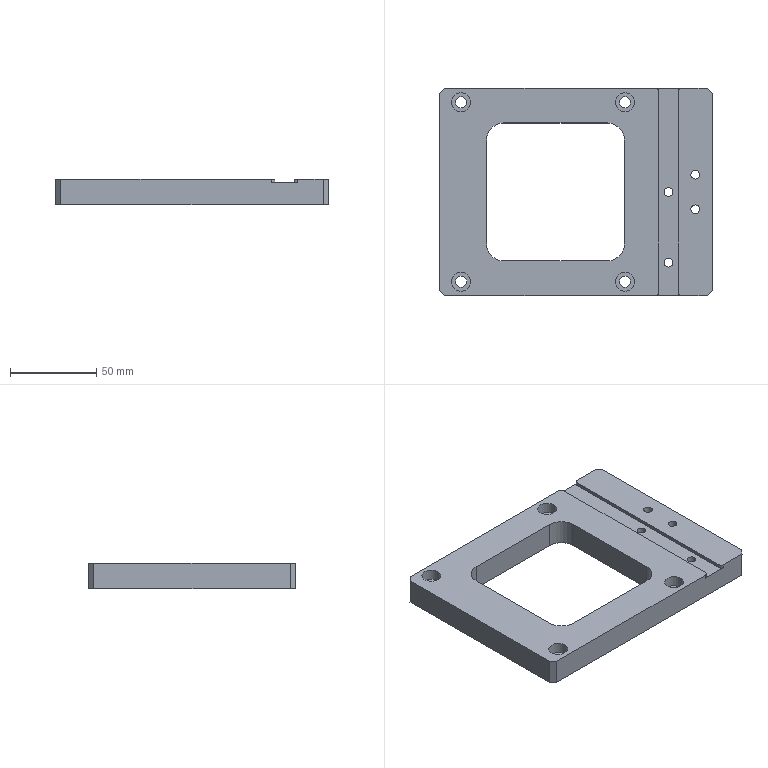Part | 1 solid | 42 faces | box 158.2 x 120 x 15 mm | volume 182408 mm3 | plane 22 | cylinder 20 | commonest cylinder face diameters 4 x4 5 x4 6.5 x4 11 x4 20 x4
STEP:
#1=CARTESIAN_POINT('',(62.95,-354.903,303.7));
#2=VERTEX_POINT('',#1);
#3=CARTESIAN_POINT('',(60.95,-352.903,303.7));
#4=VERTEX_POINT('',#3);
#5=CARTESIAN_POINT('',(60.95,-354.903,303.7));
#6=DIRECTION('',(0.,-0.000000076,1.));
#7=DIRECTION('',(0.,-1.,-0.000000076));
#8=AXIS2_PLACEMENT_3D('',#5,#6,#7);
#9=CIRCLE('',#8,2.);
#10=EDGE_CURVE('',#2,#4,#9,.T.);
#11=ORIENTED_EDGE('',*,*,#10,.F.);
#12=CARTESIAN_POINT('',(62.95,-354.903,301.7));
#13=VERTEX_POINT('',#12);
#14=CARTESIAN_POINT('',(62.95,-354.903,301.7));
#15=DIRECTION('',(0.,0.000000076,-1.));
#16=VECTOR('',#15,1000.);
#17=LINE('',#14,#16);
#18=EDGE_CURVE('',#2,#13,#17,.T.);
#19=ORIENTED_EDGE('',*,*,#18,.T.);
#20=CARTESIAN_POINT('',(60.95,-352.903,301.7));
#21=VERTEX_POINT('',#20);
#22=CARTESIAN_POINT('',(60.95,-354.903,301.7));
#23=DIRECTION('',(0.,-0.000000076,1.));
#24=DIRECTION('',(0.,1.,0.000000076));
#25=AXIS2_PLACEMENT_3D('',#22,#23,#24);
#26=CIRCLE('',#25,2.);
#27=EDGE_CURVE('',#13,#21,#26,.T.);
#28=ORIENTED_EDGE('',*,*,#27,.T.);
#29=CARTESIAN_POINT('',(60.95,-352.903,300.7));
#30=DIRECTION('',(0.,-0.000000076,1.));
#31=VECTOR('',#30,1000.);
#32=LINE('',#29,#31);
#33=EDGE_CURVE('',#21,#4,#32,.T.);
#34=ORIENTED_EDGE('',*,*,#33,.T.);
#35=EDGE_LOOP('',(#11,#19,#28,#34));
#36=FACE_BOUND('',#35,.T.);
#37=CARTESIAN_POINT('',(60.95,-354.903,300.7));
#38=DIRECTION('',(0.,0.000000076,-1.));
#39=DIRECTION('',(0.,1.,0.000000076));
#40=AXIS2_PLACEMENT_3D('',#37,#38,#39);
#41=CYLINDRICAL_SURFACE('',#40,2.);
#42=ADVANCED_FACE('',(#36),#41,.T.);
#43=ORIENTED_EDGE('',*,*,#18,.F.);
#44=CARTESIAN_POINT('',(62.95,-470.903,303.7));
#45=VERTEX_POINT('',#44);
#46=CARTESIAN_POINT('',(62.95,-546.403,303.7));
#47=DIRECTION('',(0.,-1.,-0.000000076));
#48=VECTOR('',#47,1000.);
#49=LINE('',#46,#48);
#50=EDGE_CURVE('',#2,#45,#49,.T.);
#51=ORIENTED_EDGE('',*,*,#50,.T.);
#52=CARTESIAN_POINT('',(62.95,-470.903,301.7));
#53=VERTEX_POINT('',#52);
#54=CARTESIAN_POINT('',(62.95,-470.903,301.7));
#55=DIRECTION('',(0.,-0.000000076,1.));
#56=VECTOR('',#55,1000.);
#57=LINE('',#54,#56);
#58=EDGE_CURVE('',#53,#45,#57,.T.);
#59=ORIENTED_EDGE('',*,*,#58,.F.);
#60=CARTESIAN_POINT('',(62.95,-412.903,301.7));
#61=DIRECTION('',(0.,-1.,-0.000000076));
#62=VECTOR('',#61,1000.);
#63=LINE('',#60,#62);
#64=EDGE_CURVE('',#13,#53,#63,.T.);
#65=ORIENTED_EDGE('',*,*,#64,.F.);
#66=EDGE_LOOP('',(#43,#51,#59,#65));
#67=FACE_BOUND('',#66,.T.);
#68=CARTESIAN_POINT('',(62.95,-432.903,301.7));
#69=DIRECTION('',(-1.,0.,0.));
#70=DIRECTION('',(0.,0.000000051,-1.));
#71=AXIS2_PLACEMENT_3D('',#68,#69,#70);
#72=PLANE('',#71);
#73=ADVANCED_FACE('',(#67),#72,.F.);
#74=CARTESIAN_POINT('',(60.95,-472.903,303.7));
#75=VERTEX_POINT('',#74);
#76=CARTESIAN_POINT('',(60.95,-470.903,303.7));
#77=DIRECTION('',(0.,-0.000000076,1.));
#78=DIRECTION('',(0.,-1.,-0.000000076));
#79=AXIS2_PLACEMENT_3D('',#76,#77,#78);
#80=CIRCLE('',#79,2.);
#81=EDGE_CURVE('',#75,#45,#80,.T.);
#82=ORIENTED_EDGE('',*,*,#81,.F.);
#83=CARTESIAN_POINT('',(60.95,-472.903,301.7));
#84=VERTEX_POINT('',#83);
#85=CARTESIAN_POINT('',(60.95,-472.903,288.7));
#86=DIRECTION('',(0.,0.000000076,-1.));
#87=VECTOR('',#86,1000.);
#88=LINE('',#85,#87);
#89=EDGE_CURVE('',#75,#84,#88,.T.);
#90=ORIENTED_EDGE('',*,*,#89,.T.);
#91=CARTESIAN_POINT('',(60.95,-470.903,301.7));
#92=DIRECTION('',(0.,-0.000000076,1.));
#93=DIRECTION('',(0.,1.,0.000000076));
#94=AXIS2_PLACEMENT_3D('',#91,#92,#93);
#95=CIRCLE('',#94,2.);
#96=EDGE_CURVE('',#84,#53,#95,.T.);
#97=ORIENTED_EDGE('',*,*,#96,.T.);
#98=ORIENTED_EDGE('',*,*,#58,.T.);
#99=EDGE_LOOP('',(#82,#90,#97,#98));
#100=FACE_BOUND('',#99,.T.);
#101=CARTESIAN_POINT('',(60.95,-470.903,288.7));
#102=DIRECTION('',(0.,-0.000000076,1.));
#103=DIRECTION('',(0.,-1.,-0.000000076));
#104=AXIS2_PLACEMENT_3D('',#101,#102,#103);
#105=CYLINDRICAL_SURFACE('',#104,2.);
#106=ADVANCED_FACE('',(#100),#105,.T.);
#107=ORIENTED_EDGE('',*,*,#89,.F.);
#108=CARTESIAN_POINT('',(-61.2,-472.903,303.7));
#109=VERTEX_POINT('',#108);
#110=CARTESIAN_POINT('',(3.,-472.903,303.7));
#111=DIRECTION('',(-1.,0.,0.));
#112=VECTOR('',#111,1000.);
#113=LINE('',#110,#112);
#114=EDGE_CURVE('',#75,#109,#113,.T.);
#115=ORIENTED_EDGE('',*,*,#114,.T.);
#116=CARTESIAN_POINT('',(-61.2,-472.903,288.7));
#117=VERTEX_POINT('',#116);
#118=CARTESIAN_POINT('',(-61.2,-472.903,288.7));
#119=DIRECTION('',(0.,-0.000000076,1.));
#120=VECTOR('',#119,1000.);
#121=LINE('',#118,#120);
#122=EDGE_CURVE('',#117,#109,#121,.T.);
#123=ORIENTED_EDGE('',*,*,#122,.F.);
#124=CARTESIAN_POINT('',(91.,-472.903,288.7));
#125=VERTEX_POINT('',#124);
#126=CARTESIAN_POINT('',(3.,-472.903,288.7));
#127=DIRECTION('',(1.,0.,0.));
#128=VECTOR('',#127,1000.);
#129=LINE('',#126,#128);
#130=EDGE_CURVE('',#117,#125,#129,.T.);
#131=ORIENTED_EDGE('',*,*,#130,.T.);
#132=CARTESIAN_POINT('',(91.,-472.903,303.7));
#133=VERTEX_POINT('',#132);
#134=CARTESIAN_POINT('',(91.,-472.903,288.7));
#135=DIRECTION('',(0.,0.000000076,-1.));
#136=VECTOR('',#135,1000.);
#137=LINE('',#134,#136);
#138=EDGE_CURVE('',#133,#125,#137,.T.);
#139=ORIENTED_EDGE('',*,*,#138,.F.);
#140=CARTESIAN_POINT('',(76.05,-472.903,303.7));
#141=VERTEX_POINT('',#140);
#142=CARTESIAN_POINT('',(-67.,-472.903,303.7));
#143=DIRECTION('',(1.,0.,0.));
#144=VECTOR('',#143,1000.);
#145=LINE('',#142,#144);
#146=EDGE_CURVE('',#141,#133,#145,.T.);
#147=ORIENTED_EDGE('',*,*,#146,.F.);
#148=CARTESIAN_POINT('',(76.05,-472.903,301.7));
#149=VERTEX_POINT('',#148);
#150=CARTESIAN_POINT('',(76.05,-472.903,288.7));
#151=DIRECTION('',(0.,-0.000000076,1.));
#152=VECTOR('',#151,1000.);
#153=LINE('',#150,#152);
#154=EDGE_CURVE('',#149,#141,#153,.T.);
#155=ORIENTED_EDGE('',*,*,#154,.F.);
#156=CARTESIAN_POINT('',(68.5,-472.903,301.7));
#157=DIRECTION('',(1.,0.,0.));
#158=VECTOR('',#157,1000.);
#159=LINE('',#156,#158);
#160=EDGE_CURVE('',#84,#149,#159,.T.);
#161=ORIENTED_EDGE('',*,*,#160,.F.);
#162=EDGE_LOOP('',(#107,#115,#123,#131,#139,#147,#155,#161));
#163=FACE_BOUND('',#162,.T.);
#164=CARTESIAN_POINT('',(-67.,-472.903,288.7));
#165=DIRECTION('',(0.,1.,0.000000076));
#166=DIRECTION('',(1.,0.,0.));
#167=AXIS2_PLACEMENT_3D('',#164,#165,#166);
#168=PLANE('',#167);
#169=ADVANCED_FACE('',(#163),#168,.F.);
#170=ORIENTED_EDGE('',*,*,#122,.T.);
#171=CARTESIAN_POINT('',(-64.2,-469.903,303.7));
#172=VERTEX_POINT('',#171);
#173=CARTESIAN_POINT('',(7.65,-541.753,303.7));
#174=DIRECTION('',(-0.7071,0.7071,0.000000054));
#175=VECTOR('',#174,1000.);
#176=LINE('',#173,#175);
#177=EDGE_CURVE('',#109,#172,#176,.T.);
#178=ORIENTED_EDGE('',*,*,#177,.T.);
#179=CARTESIAN_POINT('',(-64.2,-469.903,288.7));
#180=VERTEX_POINT('',#179);
#181=CARTESIAN_POINT('',(-64.2,-469.903,300.7));
#182=DIRECTION('',(0.,0.000000076,-1.));
#183=VECTOR('',#182,1000.);
#184=LINE('',#181,#183);
#185=EDGE_CURVE('',#172,#180,#184,.T.);
#186=ORIENTED_EDGE('',*,*,#185,.T.);
#187=CARTESIAN_POINT('',(-64.2,-469.903,288.7));
#188=DIRECTION('',(0.7071,-0.7071,-0.000000054));
#189=VECTOR('',#188,1000.);
#190=LINE('',#187,#189);
#191=EDGE_CURVE('',#180,#117,#190,.T.);
#192=ORIENTED_EDGE('',*,*,#191,.T.);
#193=EDGE_LOOP('',(#170,#178,#186,#192));
#194=FACE_BOUND('',#193,.T.);
#195=CARTESIAN_POINT('',(-64.2,-469.903,300.7));
#196=DIRECTION('',(0.7071,0.7071,0.000000054));
#197=DIRECTION('',(0.,-0.000000076,1.));
#198=AXIS2_PLACEMENT_3D('',#195,#196,#197);
#199=PLANE('',#198);
#200=ADVANCED_FACE('',(#194),#199,.F.);
#201=ORIENTED_EDGE('',*,*,#185,.F.);
#202=CARTESIAN_POINT('',(-64.2,-355.903,303.7));
#203=VERTEX_POINT('',#202);
#204=CARTESIAN_POINT('',(-64.2,-546.403,303.7));
#205=DIRECTION('',(0.,1.,0.000000076));
#206=VECTOR('',#205,1000.);
#207=LINE('',#204,#206);
#208=EDGE_CURVE('',#172,#203,#207,.T.);
#209=ORIENTED_EDGE('',*,*,#208,.T.);
#210=CARTESIAN_POINT('',(-64.2,-355.903,288.7));
#211=VERTEX_POINT('',#210);
#212=CARTESIAN_POINT('',(-64.2,-355.903,300.7));
#213=DIRECTION('',(0.,-0.000000076,1.));
#214=VECTOR('',#213,1000.);
#215=LINE('',#212,#214);
#216=EDGE_CURVE('',#211,#203,#215,.T.);
#217=ORIENTED_EDGE('',*,*,#216,.F.);
#218=CARTESIAN_POINT('',(-64.2,-746.403,288.7));
#219=DIRECTION('',(0.,1.,0.000000076));
#220=VECTOR('',#219,1000.);
#221=LINE('',#218,#220);
#222=EDGE_CURVE('',#180,#211,#221,.T.);
#223=ORIENTED_EDGE('',*,*,#222,.F.);
#224=EDGE_LOOP('',(#201,#209,#217,#223));
#225=FACE_BOUND('',#224,.T.);
#226=CARTESIAN_POINT('',(-64.2,-746.403,300.7));
#227=DIRECTION('',(1.,0.,0.));
#228=DIRECTION('',(0.,-0.000000076,1.));
#229=AXIS2_PLACEMENT_3D('',#226,#227,#228);
#230=PLANE('',#229);
#231=ADVANCED_FACE('',(#225),#230,.F.);
#232=ORIENTED_EDGE('',*,*,#216,.T.);
#233=CARTESIAN_POINT('',(-61.2,-352.903,303.7));
#234=VERTEX_POINT('',#233);
#235=CARTESIAN_POINT('',(-125.85,-417.553,303.7));
#236=DIRECTION('',(0.7071,0.7071,0.000000054));
#237=VECTOR('',#236,1000.);
#238=LINE('',#235,#237);
#239=EDGE_CURVE('',#203,#234,#238,.T.);
#240=ORIENTED_EDGE('',*,*,#239,.T.);
#241=CARTESIAN_POINT('',(-61.2,-352.903,288.7));
#242=VERTEX_POINT('',#241);
#243=CARTESIAN_POINT('',(-61.2,-352.903,300.7));
#244=DIRECTION('',(0.,0.000000076,-1.));
#245=VECTOR('',#244,1000.);
#246=LINE('',#243,#245);
#247=EDGE_CURVE('',#234,#242,#246,.T.);
#248=ORIENTED_EDGE('',*,*,#247,.T.);
#249=CARTESIAN_POINT('',(-64.2,-355.903,288.7));
#250=DIRECTION('',(-0.7071,-0.7071,-0.000000054));
#251=VECTOR('',#250,1000.);
#252=LINE('',#249,#251);
#253=EDGE_CURVE('',#242,#211,#252,.T.);
#254=ORIENTED_EDGE('',*,*,#253,.T.);
#255=EDGE_LOOP('',(#232,#240,#248,#254));
#256=FACE_BOUND('',#255,.T.);
#257=CARTESIAN_POINT('',(-64.2,-355.903,300.7));
#258=DIRECTION('',(0.7071,-0.7071,-0.000000054));
#259=DIRECTION('',(0.,0.000000076,-1.));
#260=AXIS2_PLACEMENT_3D('',#257,#258,#259);
#261=PLANE('',#260);
#262=ADVANCED_FACE('',(#256),#261,.F.);
#263=ORIENTED_EDGE('',*,*,#247,.F.);
#264=CARTESIAN_POINT('',(3.,-352.903,303.7));
#265=DIRECTION('',(1.,0.,0.));
#266=VECTOR('',#265,1000.);
#267=LINE('',#264,#266);
#268=EDGE_CURVE('',#234,#4,#267,.T.);
#269=ORIENTED_EDGE('',*,*,#268,.T.);
#270=ORIENTED_EDGE('',*,*,#33,.F.);
#271=CARTESIAN_POINT('',(76.05,-352.903,301.7));
#272=VERTEX_POINT('',#271);
#273=CARTESIAN_POINT('',(68.5,-352.903,301.7));
#274=DIRECTION('',(-1.,0.,0.));
#275=VECTOR('',#274,1000.);
#276=LINE('',#273,#275);
#277=EDGE_CURVE('',#272,#21,#276,.T.);
#278=ORIENTED_EDGE('',*,*,#277,.F.);
#279=CARTESIAN_POINT('',(76.05,-352.903,303.7));
#280=VERTEX_POINT('',#279);
#281=CARTESIAN_POINT('',(76.05,-352.903,300.7));
#282=DIRECTION('',(0.,0.000000076,-1.));
#283=VECTOR('',#282,1000.);
#284=LINE('',#281,#283);
#285=EDGE_CURVE('',#280,#272,#284,.T.);
#286=ORIENTED_EDGE('',*,*,#285,.F.);
#287=CARTESIAN_POINT('',(91.,-352.903,303.7));
#288=VERTEX_POINT('',#287);
#289=CARTESIAN_POINT('',(-67.,-352.903,303.7));
#290=DIRECTION('',(-1.,0.,0.));
#291=VECTOR('',#290,1000.);
#292=LINE('',#289,#291);
#293=EDGE_CURVE('',#288,#280,#292,.T.);
#294=ORIENTED_EDGE('',*,*,#293,.F.);
#295=CARTESIAN_POINT('',(91.,-352.903,288.7));
#296=VERTEX_POINT('',#295);
#297=CARTESIAN_POINT('',(91.,-352.903,300.7));
#298=DIRECTION('',(0.,-0.000000076,1.));
#299=VECTOR('',#298,1000.);
#300=LINE('',#297,#299);
#301=EDGE_CURVE('',#296,#288,#300,.T.);
#302=ORIENTED_EDGE('',*,*,#301,.F.);
#303=CARTESIAN_POINT('',(-67.,-352.903,288.7));
#304=DIRECTION('',(1.,0.,0.));
#305=VECTOR('',#304,1000.);
#306=LINE('',#303,#305);
#307=EDGE_CURVE('',#242,#296,#306,.T.);
#308=ORIENTED_EDGE('',*,*,#307,.F.);
#309=EDGE_LOOP('',(#263,#269,#270,#278,#286,#294,#302,#308));
#310=FACE_BOUND('',#309,.T.);
#311=CARTESIAN_POINT('',(-67.,-352.903,300.7));
#312=DIRECTION('',(0.,-1.,-0.000000076));
#313=DIRECTION('',(0.,0.000000076,-1.));
#314=AXIS2_PLACEMENT_3D('',#311,#312,#313);
#315=PLANE('',#314);
#316=ADVANCED_FACE('',(#310),#315,.F.);
#317=CARTESIAN_POINT('',(84.,-405.403,303.7));
#318=VERTEX_POINT('',#317);
#319=CARTESIAN_POINT('',(84.,-402.903,303.7));
#320=DIRECTION('',(0.,0.000000076,-1.));
#321=DIRECTION('',(0.,-1.,-0.000000076));
#322=AXIS2_PLACEMENT_3D('',#319,#320,#321);
#323=CIRCLE('',#322,2.5);
#324=EDGE_CURVE('',#318,#318,#323,.T.);
#325=ORIENTED_EDGE('',*,*,#324,.T.);
#326=EDGE_LOOP('',(#325));
#327=FACE_BOUND('',#326,.T.);
#328=CARTESIAN_POINT('',(84.,-425.403,303.7));
#329=VERTEX_POINT('',#328);
#330=CARTESIAN_POINT('',(84.,-422.903,303.7));
#331=DIRECTION('',(0.,0.000000076,-1.));
#332=DIRECTION('',(0.,-1.,-0.000000076));
#333=AXIS2_PLACEMENT_3D('',#330,#331,#332);
#334=CIRCLE('',#333,2.5);
#335=EDGE_CURVE('',#329,#329,#334,.T.);
#336=ORIENTED_EDGE('',*,*,#335,.T.);
#337=EDGE_LOOP('',(#336));
#338=FACE_BOUND('',#337,.T.);
#339=CARTESIAN_POINT('',(74.05,-354.903,303.7));
#340=VERTEX_POINT('',#339);
#341=CARTESIAN_POINT('',(76.05,-354.903,303.7));
#342=DIRECTION('',(0.,-0.000000076,1.));
#343=DIRECTION('',(0.,-1.,-0.000000076));
#344=AXIS2_PLACEMENT_3D('',#341,#342,#343);
#345=CIRCLE('',#344,2.);
#346=EDGE_CURVE('',#340,#280,#345,.F.);
#347=ORIENTED_EDGE('',*,*,#346,.F.);
#348=CARTESIAN_POINT('',(74.05,-470.903,303.7));
#349=VERTEX_POINT('',#348);
#350=CARTESIAN_POINT('',(74.05,-432.903,303.7));
#351=DIRECTION('',(0.,-1.,-0.000000076));
#352=VECTOR('',#351,1000.);
#353=LINE('',#350,#352);
#354=EDGE_CURVE('',#340,#349,#353,.T.);
#355=ORIENTED_EDGE('',*,*,#354,.T.);
#356=CARTESIAN_POINT('',(76.05,-470.903,303.7));
#357=DIRECTION('',(0.,-0.000000076,1.));
#358=DIRECTION('',(0.,-1.,-0.000000076));
#359=AXIS2_PLACEMENT_3D('',#356,#357,#358);
#360=CIRCLE('',#359,2.);
#361=EDGE_CURVE('',#141,#349,#360,.F.);
#362=ORIENTED_EDGE('',*,*,#361,.F.);
#363=ORIENTED_EDGE('',*,*,#146,.T.);
#364=CARTESIAN_POINT('',(94.,-469.903,303.7));
#365=VERTEX_POINT('',#364);
#366=CARTESIAN_POINT('',(91.,-472.903,303.7));
#367=DIRECTION('',(0.7071,0.7071,0.000000054));
#368=VECTOR('',#367,1000.);
#369=LINE('',#366,#368);
#370=EDGE_CURVE('',#133,#365,#369,.T.);
#371=ORIENTED_EDGE('',*,*,#370,.T.);
#372=CARTESIAN_POINT('',(94.,-355.903,303.7));
#373=VERTEX_POINT('',#372);
#374=CARTESIAN_POINT('',(94.,-450.403,303.7));
#375=DIRECTION('',(0.,1.,0.000000076));
#376=VECTOR('',#375,1000.);
#377=LINE('',#374,#376);
#378=EDGE_CURVE('',#365,#373,#377,.T.);
#379=ORIENTED_EDGE('',*,*,#378,.T.);
#380=CARTESIAN_POINT('',(91.,-352.903,303.7));
#381=DIRECTION('',(-0.7071,0.7071,0.000000054));
#382=VECTOR('',#381,1000.);
#383=LINE('',#380,#382);
#384=EDGE_CURVE('',#373,#288,#383,.T.);
#385=ORIENTED_EDGE('',*,*,#384,.T.);
#386=ORIENTED_EDGE('',*,*,#293,.T.);
#387=EDGE_LOOP('',(#347,#355,#362,#363,#371,#379,#385,#386));
#388=FACE_BOUND('',#387,.T.);
#389=CARTESIAN_POINT('',(3.,-546.403,303.7));
#390=DIRECTION('',(0.,-0.000000076,1.));
#391=DIRECTION('',(0.,-1.,-0.000000076));
#392=AXIS2_PLACEMENT_3D('',#389,#390,#391);
#393=PLANE('',#392);
#394=ADVANCED_FACE('',(#327,#338,#388),#393,.T.);
#395=CARTESIAN_POINT('',(84.,-405.403,288.7));
#396=VERTEX_POINT('',#395);
#397=CARTESIAN_POINT('',(84.,-402.903,288.7));
#398=DIRECTION('',(0.,0.000000076,-1.));
#399=DIRECTION('',(0.,-1.,-0.000000076));
#400=AXIS2_PLACEMENT_3D('',#397,#398,#399);
#401=CIRCLE('',#400,2.5);
#402=EDGE_CURVE('',#396,#396,#401,.T.);
#403=ORIENTED_EDGE('',*,*,#402,.T.);
#404=EDGE_LOOP('',(#403));
#405=FACE_BOUND('',#404,.T.);
#406=ORIENTED_EDGE('',*,*,#324,.F.);
#407=EDGE_LOOP('',(#406));
#408=FACE_BOUND('',#407,.T.);
#409=CARTESIAN_POINT('',(84.,-402.903,296.2));
#410=DIRECTION('',(0.,0.000000076,-1.));
#411=DIRECTION('',(1.,0.,0.));
#412=AXIS2_PLACEMENT_3D('',#409,#410,#411);
#413=CYLINDRICAL_SURFACE('',#412,2.5);
#414=ADVANCED_FACE('',(#405,#408),#413,.F.);
#415=CARTESIAN_POINT('',(84.,-425.403,288.7));
#416=VERTEX_POINT('',#415);
#417=CARTESIAN_POINT('',(84.,-422.903,288.7));
#418=DIRECTION('',(0.,0.000000076,-1.));
#419=DIRECTION('',(0.,-1.,-0.000000076));
#420=AXIS2_PLACEMENT_3D('',#417,#418,#419);
#421=CIRCLE('',#420,2.5);
#422=EDGE_CURVE('',#416,#416,#421,.T.);
#423=ORIENTED_EDGE('',*,*,#422,.T.);
#424=EDGE_LOOP('',(#423));
#425=FACE_BOUND('',#424,.T.);
#426=ORIENTED_EDGE('',*,*,#335,.F.);
#427=EDGE_LOOP('',(#426));
#428=FACE_BOUND('',#427,.T.);
#429=CARTESIAN_POINT('',(84.,-422.903,296.2));
#430=DIRECTION('',(0.,0.000000076,-1.));
#431=DIRECTION('',(1.,0.,0.));
#432=AXIS2_PLACEMENT_3D('',#429,#430,#431);
#433=CYLINDRICAL_SURFACE('',#432,2.5);
#434=ADVANCED_FACE('',(#425,#428),#433,.F.);
#435=ORIENTED_EDGE('',*,*,#154,.T.);
#436=ORIENTED_EDGE('',*,*,#361,.T.);
#437=CARTESIAN_POINT('',(74.05,-470.903,301.7));
#438=VERTEX_POINT('',#437);
#439=CARTESIAN_POINT('',(74.05,-470.903,301.7));
#440=DIRECTION('',(0.,0.000000076,-1.));
#441=VECTOR('',#440,1000.);
#442=LINE('',#439,#441);
#443=EDGE_CURVE('',#349,#438,#442,.T.);
#444=ORIENTED_EDGE('',*,*,#443,.T.);
#445=CARTESIAN_POINT('',(76.05,-470.903,301.7));
#446=DIRECTION('',(0.,-0.000000076,1.));
#447=DIRECTION('',(0.,1.,0.000000076));
#448=AXIS2_PLACEMENT_3D('',#445,#446,#447);
#449=CIRCLE('',#448,2.);
#450=EDGE_CURVE('',#438,#149,#449,.T.);
#451=ORIENTED_EDGE('',*,*,#450,.T.);
#452=EDGE_LOOP('',(#435,#436,#444,#451));
#453=FACE_BOUND('',#452,.T.);
#454=CARTESIAN_POINT('',(76.05,-470.903,288.7));
#455=DIRECTION('',(0.,0.000000076,-1.));
#456=DIRECTION('',(0.,1.,0.000000076));
#457=AXIS2_PLACEMENT_3D('',#454,#455,#456);
#458=CYLINDRICAL_SURFACE('',#457,2.);
#459=ADVANCED_FACE('',(#453),#458,.T.);
#460=CARTESIAN_POINT('',(74.05,-354.903,301.7));
#461=VERTEX_POINT('',#460);
#462=CARTESIAN_POINT('',(74.05,-354.903,301.7));
#463=DIRECTION('',(0.,-0.000000076,1.));
#464=VECTOR('',#463,1000.);
#465=LINE('',#462,#464);
#466=EDGE_CURVE('',#461,#340,#465,.T.);
#467=ORIENTED_EDGE('',*,*,#466,.T.);
#468=ORIENTED_EDGE('',*,*,#346,.T.);
#469=ORIENTED_EDGE('',*,*,#285,.T.);
#470=CARTESIAN_POINT('',(76.05,-354.903,301.7));
#471=DIRECTION('',(0.,-0.000000076,1.));
#472=DIRECTION('',(0.,1.,0.000000076));
#473=AXIS2_PLACEMENT_3D('',#470,#471,#472);
#474=CIRCLE('',#473,2.);
#475=EDGE_CURVE('',#272,#461,#474,.T.);
#476=ORIENTED_EDGE('',*,*,#475,.T.);
#477=EDGE_LOOP('',(#467,#468,#469,#476));
#478=FACE_BOUND('',#477,.T.);
#479=CARTESIAN_POINT('',(76.05,-354.903,300.7));
#480=DIRECTION('',(0.,-0.000000076,1.));
#481=DIRECTION('',(0.,-1.,-0.000000076));
#482=AXIS2_PLACEMENT_3D('',#479,#480,#481);
#483=CYLINDRICAL_SURFACE('',#482,2.);
#484=ADVANCED_FACE('',(#478),#483,.T.);
#485=CARTESIAN_POINT('',(33.,-452.903,288.7));
#486=VERTEX_POINT('',#485);
#487=CARTESIAN_POINT('',(33.,-452.903,303.7));
#488=VERTEX_POINT('',#487);
#489=CARTESIAN_POINT('',(33.,-452.903,296.2));
#490=DIRECTION('',(0.,-0.000000076,1.));
#491=VECTOR('',#490,1000.);
#492=LINE('',#489,#491);
#493=EDGE_CURVE('',#486,#488,#492,.T.);
#494=ORIENTED_EDGE('',*,*,#493,.T.);
#495=CARTESIAN_POINT('',(43.,-442.903,303.7));
#496=VERTEX_POINT('',#495);
#497=CARTESIAN_POINT('',(33.,-442.903,303.7));
#498=DIRECTION('',(0.,-0.000000076,1.));
#499=DIRECTION('',(0.,-1.,-0.000000076));
#500=AXIS2_PLACEMENT_3D('',#497,#498,#499);
#501=CIRCLE('',#500,10.);
#502=EDGE_CURVE('',#488,#496,#501,.T.);
#503=ORIENTED_EDGE('',*,*,#502,.T.);
#504=CARTESIAN_POINT('',(43.,-442.903,288.7));
#505=VERTEX_POINT('',#504);
#506=CARTESIAN_POINT('',(43.,-442.903,303.7));
#507=DIRECTION('',(0.,0.000000076,-1.));
#508=VECTOR('',#507,1000.);
#509=LINE('',#506,#508);
#510=EDGE_CURVE('',#496,#505,#509,.T.);
#511=ORIENTED_EDGE('',*,*,#510,.T.);
#512=CARTESIAN_POINT('',(33.,-442.903,288.7));
#513=DIRECTION('',(0.,0.000000076,-1.));
#514=DIRECTION('',(0.,-1.,-0.000000076));
#515=AXIS2_PLACEMENT_3D('',#512,#513,#514);
#516=CIRCLE('',#515,10.);
#517=EDGE_CURVE('',#505,#486,#516,.T.);
#518=ORIENTED_EDGE('',*,*,#517,.T.);
#519=EDGE_LOOP('',(#494,#503,#511,#518));
#520=FACE_BOUND('',#519,.T.);
#521=CARTESIAN_POINT('',(33.,-442.903,303.7));
#522=DIRECTION('',(0.,-0.000000076,1.));
#523=DIRECTION('',(0.,-1.,-0.000000076));
#524=AXIS2_PLACEMENT_3D('',#521,#522,#523);
#525=CYLINDRICAL_SURFACE('',#524,10.);
#526=ADVANCED_FACE('',(#520),#525,.F.);
#527=CARTESIAN_POINT('',(-37.,-442.903,288.7));
#528=VERTEX_POINT('',#527);
#529=CARTESIAN_POINT('',(-37.,-442.903,303.7));
#530=VERTEX_POINT('',#529);
#531=CARTESIAN_POINT('',(-37.,-442.903,288.7));
#532=DIRECTION('',(0.,-0.000000076,1.));
#533=VECTOR('',#532,1000.);
#534=LINE('',#531,#533);
#535=EDGE_CURVE('',#528,#530,#534,.T.);
#536=ORIENTED_EDGE('',*,*,#535,.T.);
#537=CARTESIAN_POINT('',(-27.,-452.903,303.7));
#538=VERTEX_POINT('',#537);
#539=CARTESIAN_POINT('',(-27.,-442.903,303.7));
#540=DIRECTION('',(0.,-0.000000076,1.));
#541=DIRECTION('',(0.,-1.,-0.000000076));
#542=AXIS2_PLACEMENT_3D('',#539,#540,#541);
#543=CIRCLE('',#542,10.);
#544=EDGE_CURVE('',#530,#538,#543,.T.);
#545=ORIENTED_EDGE('',*,*,#544,.T.);
#546=CARTESIAN_POINT('',(-27.,-452.903,288.7));
#547=VERTEX_POINT('',#546);
#548=CARTESIAN_POINT('',(-27.,-452.903,303.7));
#549=DIRECTION('',(0.,0.000000076,-1.));
#550=VECTOR('',#549,1000.);
#551=LINE('',#548,#550);
#552=EDGE_CURVE('',#538,#547,#551,.T.);
#553=ORIENTED_EDGE('',*,*,#552,.T.);
#554=CARTESIAN_POINT('',(-27.,-442.903,288.7));
#555=DIRECTION('',(0.,0.000000076,-1.));
#556=DIRECTION('',(0.,-1.,-0.000000076));
#557=AXIS2_PLACEMENT_3D('',#554,#555,#556);
#558=CIRCLE('',#557,10.);
#559=EDGE_CURVE('',#547,#528,#558,.T.);
#560=ORIENTED_EDGE('',*,*,#559,.T.);
#561=EDGE_LOOP('',(#536,#545,#553,#560));
#562=FACE_BOUND('',#561,.T.);
#563=CARTESIAN_POINT('',(-27.,-442.903,296.2));
#564=DIRECTION('',(0.,0.000000076,-1.));
#565=DIRECTION('',(0.,1.,0.000000076));
#566=AXIS2_PLACEMENT_3D('',#563,#564,#565);
#567=CYLINDRICAL_SURFACE('',#566,10.);
#568=ADVANCED_FACE('',(#562),#567,.F.);
#569=CARTESIAN_POINT('',(43.,-382.903,288.7));
#570=VERTEX_POINT('',#569);
#571=CARTESIAN_POINT('',(43.,-382.903,303.7));
#572=VERTEX_POINT('',#571);
#573=CARTESIAN_POINT('',(43.,-382.903,303.7));
#574=DIRECTION('',(0.,-0.000000076,1.));
#575=VECTOR('',#574,1000.);
#576=LINE('',#573,#575);
#577=EDGE_CURVE('',#570,#572,#576,.T.);
#578=ORIENTED_EDGE('',*,*,#577,.T.);
#579=CARTESIAN_POINT('',(33.,-372.903,303.7));
#580=VERTEX_POINT('',#579);
#581=CARTESIAN_POINT('',(33.,-382.903,303.7));
#582=DIRECTION('',(0.,-0.000000076,1.));
#583=DIRECTION('',(0.,-1.,-0.000000076));
#584=AXIS2_PLACEMENT_3D('',#581,#582,#583);
#585=CIRCLE('',#584,10.);
#586=EDGE_CURVE('',#572,#580,#585,.T.);
#587=ORIENTED_EDGE('',*,*,#586,.T.);
#588=CARTESIAN_POINT('',(33.,-372.903,288.7));
#589=VERTEX_POINT('',#588);
#590=CARTESIAN_POINT('',(33.,-372.903,296.2));
#591=DIRECTION('',(0.,0.000000076,-1.));
#592=VECTOR('',#591,1000.);
#593=LINE('',#590,#592);
#594=EDGE_CURVE('',#580,#589,#593,.T.);
#595=ORIENTED_EDGE('',*,*,#594,.T.);
#596=CARTESIAN_POINT('',(33.,-382.903,288.7));
#597=DIRECTION('',(0.,0.000000076,-1.));
#598=DIRECTION('',(0.,-1.,-0.000000076));
#599=AXIS2_PLACEMENT_3D('',#596,#597,#598);
#600=CIRCLE('',#599,10.);
#601=EDGE_CURVE('',#589,#570,#600,.T.);
#602=ORIENTED_EDGE('',*,*,#601,.T.);
#603=EDGE_LOOP('',(#578,#587,#595,#602));
#604=FACE_BOUND('',#603,.T.);
#605=CARTESIAN_POINT('',(33.,-382.903,303.7));
#606=DIRECTION('',(0.,0.000000076,-1.));
#607=DIRECTION('',(0.,1.,0.000000076));
#608=AXIS2_PLACEMENT_3D('',#605,#606,#607);
#609=CYLINDRICAL_SURFACE('',#608,10.);
#610=ADVANCED_FACE('',(#604),#609,.F.);
#611=CARTESIAN_POINT('',(-27.,-372.903,288.7));
#612=VERTEX_POINT('',#611);
#613=CARTESIAN_POINT('',(-27.,-372.903,303.7));
#614=VERTEX_POINT('',#613);
#615=CARTESIAN_POINT('',(-27.,-372.903,288.7));
#616=DIRECTION('',(0.,-0.000000076,1.));
#617=VECTOR('',#616,1000.);
#618=LINE('',#615,#617);
#619=EDGE_CURVE('',#612,#614,#618,.T.);
#620=ORIENTED_EDGE('',*,*,#619,.T.);
#621=CARTESIAN_POINT('',(-37.,-382.903,303.7));
#622=VERTEX_POINT('',#621);
#623=CARTESIAN_POINT('',(-27.,-382.903,303.7));
#624=DIRECTION('',(0.,-0.000000076,1.));
#625=DIRECTION('',(0.,-1.,-0.000000076));
#626=AXIS2_PLACEMENT_3D('',#623,#624,#625);
#627=CIRCLE('',#626,10.);
#628=EDGE_CURVE('',#614,#622,#627,.T.);
#629=ORIENTED_EDGE('',*,*,#628,.T.);
#630=CARTESIAN_POINT('',(-37.,-382.903,288.7));
#631=VERTEX_POINT('',#630);
#632=CARTESIAN_POINT('',(-37.,-382.903,303.7));
#633=DIRECTION('',(0.,0.000000076,-1.));
#634=VECTOR('',#633,1000.);
#635=LINE('',#632,#634);
#636=EDGE_CURVE('',#622,#631,#635,.T.);
#637=ORIENTED_EDGE('',*,*,#636,.T.);
#638=CARTESIAN_POINT('',(-27.,-382.903,288.7));
#639=DIRECTION('',(0.,0.000000076,-1.));
#640=DIRECTION('',(0.,-1.,-0.000000076));
#641=AXIS2_PLACEMENT_3D('',#638,#639,#640);
#642=CIRCLE('',#641,10.);
#643=EDGE_CURVE('',#631,#612,#642,.T.);
#644=ORIENTED_EDGE('',*,*,#643,.T.);
#645=EDGE_LOOP('',(#620,#629,#637,#644));
#646=FACE_BOUND('',#645,.T.);
#647=CARTESIAN_POINT('',(-27.,-382.903,296.2));
#648=DIRECTION('',(0.,0.000000076,-1.));
#649=DIRECTION('',(0.,1.,0.000000076));
#650=AXIS2_PLACEMENT_3D('',#647,#648,#649);
#651=CYLINDRICAL_SURFACE('',#650,10.);
#652=ADVANCED_FACE('',(#646),#651,.F.);
#653=ORIENTED_EDGE('',*,*,#636,.F.);
#654=CARTESIAN_POINT('',(-37.,-546.403,303.7));
#655=DIRECTION('',(0.,-1.,-0.000000076));
#656=VECTOR('',#655,1000.);
#657=LINE('',#654,#656);
#658=EDGE_CURVE('',#622,#530,#657,.T.);
#659=ORIENTED_EDGE('',*,*,#658,.T.);
#660=ORIENTED_EDGE('',*,*,#535,.F.);
#661=CARTESIAN_POINT('',(-37.,-546.403,288.7));
#662=DIRECTION('',(0.,1.,0.000000076));
#663=VECTOR('',#662,1000.);
#664=LINE('',#661,#663);
#665=EDGE_CURVE('',#528,#631,#664,.T.);
#666=ORIENTED_EDGE('',*,*,#665,.T.);
#667=EDGE_LOOP('',(#653,#659,#660,#666));
#668=FACE_BOUND('',#667,.T.);
#669=CARTESIAN_POINT('',(-37.,-412.903,296.2));
#670=DIRECTION('',(-1.,0.,0.));
#671=DIRECTION('',(0.,-0.000000051,1.));
#672=AXIS2_PLACEMENT_3D('',#669,#670,#671);
#673=PLANE('',#672);
#674=ADVANCED_FACE('',(#668),#673,.F.);
#675=ORIENTED_EDGE('',*,*,#510,.F.);
#676=CARTESIAN_POINT('',(43.,-546.403,303.7));
#677=DIRECTION('',(0.,-1.,-0.000000076));
#678=VECTOR('',#677,1000.);
#679=LINE('',#676,#678);
#680=EDGE_CURVE('',#572,#496,#679,.T.);
#681=ORIENTED_EDGE('',*,*,#680,.F.);
#682=ORIENTED_EDGE('',*,*,#577,.F.);
#683=CARTESIAN_POINT('',(43.,-546.403,288.7));
#684=DIRECTION('',(0.,-1.,-0.000000076));
#685=VECTOR('',#684,1000.);
#686=LINE('',#683,#685);
#687=EDGE_CURVE('',#570,#505,#686,.T.);
#688=ORIENTED_EDGE('',*,*,#687,.T.);
#689=EDGE_LOOP('',(#675,#681,#682,#688));
#690=FACE_BOUND('',#689,.T.);
#691=CARTESIAN_POINT('',(43.,-464.903,303.7));
#692=DIRECTION('',(-1.,0.,0.));
#693=DIRECTION('',(0.,-0.000000051,1.));
#694=AXIS2_PLACEMENT_3D('',#691,#692,#693);
#695=PLANE('',#694);
#696=ADVANCED_FACE('',(#690),#695,.T.);
#697=CARTESIAN_POINT('',(68.5,-415.403,288.7));
#698=VERTEX_POINT('',#697);
#699=CARTESIAN_POINT('',(68.5,-412.903,288.7));
#700=DIRECTION('',(0.,0.000000076,-1.));
#701=DIRECTION('',(0.,-1.,-0.000000076));
#702=AXIS2_PLACEMENT_3D('',#699,#700,#701);
#703=CIRCLE('',#702,2.5);
#704=EDGE_CURVE('',#698,#698,#703,.T.);
#705=ORIENTED_EDGE('',*,*,#704,.T.);
#706=EDGE_LOOP('',(#705));
#707=FACE_BOUND('',#706,.T.);
#708=CARTESIAN_POINT('',(68.5,-410.403,301.7));
#709=VERTEX_POINT('',#708);
#710=CARTESIAN_POINT('',(68.5,-412.903,301.7));
#711=DIRECTION('',(0.,-0.000000076,1.));
#712=DIRECTION('',(0.,1.,0.000000076));
#713=AXIS2_PLACEMENT_3D('',#710,#711,#712);
#714=CIRCLE('',#713,2.5);
#715=EDGE_CURVE('',#709,#709,#714,.T.);
#716=ORIENTED_EDGE('',*,*,#715,.T.);
#717=EDGE_LOOP('',(#716));
#718=FACE_BOUND('',#717,.T.);
#719=CARTESIAN_POINT('',(68.5,-412.903,295.2));
#720=DIRECTION('',(0.,0.000000076,-1.));
#721=DIRECTION('',(1.,0.,0.));
#722=AXIS2_PLACEMENT_3D('',#719,#720,#721);
#723=CYLINDRICAL_SURFACE('',#722,2.5);
#724=ADVANCED_FACE('',(#707,#718),#723,.F.);
#725=CARTESIAN_POINT('',(43.3,-364.153,288.7));
#726=VERTEX_POINT('',#725);
#727=CARTESIAN_POINT('',(43.3,-360.903,288.7));
#728=DIRECTION('',(0.,0.000000076,-1.));
#729=DIRECTION('',(0.,-1.,-0.000000076));
#730=AXIS2_PLACEMENT_3D('',#727,#728,#729);
#731=CIRCLE('',#730,3.25);
#732=EDGE_CURVE('',#726,#726,#731,.T.);
#733=ORIENTED_EDGE('',*,*,#732,.T.);
#734=EDGE_LOOP('',(#733));
#735=FACE_BOUND('',#734,.T.);
#736=CARTESIAN_POINT('',(43.3,-357.653,297.2));
#737=VERTEX_POINT('',#736);
#738=CARTESIAN_POINT('',(43.3,-360.903,297.2));
#739=DIRECTION('',(0.,0.000000076,-1.));
#740=DIRECTION('',(0.,1.,0.000000076));
#741=AXIS2_PLACEMENT_3D('',#738,#739,#740);
#742=CIRCLE('',#741,3.25);
#743=EDGE_CURVE('',#737,#737,#742,.T.);
#744=ORIENTED_EDGE('',*,*,#743,.F.);
#745=EDGE_LOOP('',(#744));
#746=FACE_BOUND('',#745,.T.);
#747=CARTESIAN_POINT('',(43.3,-360.903,243.7));
#748=DIRECTION('',(0.,0.000000076,-1.));
#749=DIRECTION('',(0.,1.,0.000000076));
#750=AXIS2_PLACEMENT_3D('',#747,#748,#749);
#751=CYLINDRICAL_SURFACE('',#750,3.25);
#752=ADVANCED_FACE('',(#735,#746),#751,.F.);
#753=CARTESIAN_POINT('',(-51.7,-364.153,288.7));
#754=VERTEX_POINT('',#753);
#755=CARTESIAN_POINT('',(-51.7,-360.903,288.7));
#756=DIRECTION('',(0.,0.000000076,-1.));
#757=DIRECTION('',(0.,-1.,-0.000000076));
#758=AXIS2_PLACEMENT_3D('',#755,#756,#757);
#759=CIRCLE('',#758,3.25);
#760=EDGE_CURVE('',#754,#754,#759,.T.);
#761=ORIENTED_EDGE('',*,*,#760,.T.);
#762=EDGE_LOOP('',(#761));
#763=FACE_BOUND('',#762,.T.);
#764=CARTESIAN_POINT('',(-51.7,-357.653,297.2));
#765=VERTEX_POINT('',#764);
#766=CARTESIAN_POINT('',(-51.7,-360.903,297.2));
#767=DIRECTION('',(0.,0.000000076,-1.));
#768=DIRECTION('',(0.,1.,0.000000076));
#769=AXIS2_PLACEMENT_3D('',#766,#767,#768);
#770=CIRCLE('',#769,3.25);
#771=EDGE_CURVE('',#765,#765,#770,.T.);
#772=ORIENTED_EDGE('',*,*,#771,.F.);
#773=EDGE_LOOP('',(#772));
#774=FACE_BOUND('',#773,.T.);
#775=CARTESIAN_POINT('',(-51.7,-360.903,243.7));
#776=DIRECTION('',(0.,0.000000076,-1.));
#777=DIRECTION('',(0.,1.,0.000000076));
#778=AXIS2_PLACEMENT_3D('',#775,#776,#777);
#779=CYLINDRICAL_SURFACE('',#778,3.25);
#780=ADVANCED_FACE('',(#763,#774),#779,.F.);
#781=ORIENTED_EDGE('',*,*,#384,.F.);
#782=CARTESIAN_POINT('',(94.,-355.903,288.7));
#783=VERTEX_POINT('',#782);
#784=CARTESIAN_POINT('',(94.,-355.903,391.2));
#785=DIRECTION('',(0.,0.000000076,-1.));
#786=VECTOR('',#785,1000.);
#787=LINE('',#784,#786);
#788=EDGE_CURVE('',#373,#783,#787,.T.);
#789=ORIENTED_EDGE('',*,*,#788,.T.);
#790=CARTESIAN_POINT('',(91.,-352.903,288.7));
#791=DIRECTION('',(-0.7071,0.7071,0.000000054));
#792=VECTOR('',#791,1000.);
#793=LINE('',#790,#792);
#794=EDGE_CURVE('',#783,#296,#793,.T.);
#795=ORIENTED_EDGE('',*,*,#794,.T.);
#796=ORIENTED_EDGE('',*,*,#301,.T.);
#797=EDGE_LOOP('',(#781,#789,#795,#796));
#798=FACE_BOUND('',#797,.T.);
#799=CARTESIAN_POINT('',(91.,-352.903,300.7));
#800=DIRECTION('',(-0.7071,-0.7071,-0.000000054));
#801=DIRECTION('',(0.,0.000000076,-1.));
#802=AXIS2_PLACEMENT_3D('',#799,#800,#801);
#803=PLANE('',#802);
#804=ADVANCED_FACE('',(#798),#803,.F.);
#805=CARTESIAN_POINT('',(43.3,-355.403,297.2));
#806=VERTEX_POINT('',#805);
#807=CARTESIAN_POINT('',(43.3,-360.903,297.2));
#808=DIRECTION('',(0.,0.000000076,-1.));
#809=DIRECTION('',(0.,1.,0.000000076));
#810=AXIS2_PLACEMENT_3D('',#807,#808,#809);
#811=CIRCLE('',#810,5.5);
#812=EDGE_CURVE('',#806,#806,#811,.T.);
#813=ORIENTED_EDGE('',*,*,#812,.T.);
#814=EDGE_LOOP('',(#813));
#815=FACE_BOUND('',#814,.T.);
#816=CARTESIAN_POINT('',(43.3,-366.403,303.7));
#817=VERTEX_POINT('',#816);
#818=CARTESIAN_POINT('',(43.3,-360.903,303.7));
#819=DIRECTION('',(0.,-0.000000076,1.));
#820=DIRECTION('',(0.,-1.,-0.000000076));
#821=AXIS2_PLACEMENT_3D('',#818,#819,#820);
#822=CIRCLE('',#821,5.5);
#823=EDGE_CURVE('',#817,#817,#822,.T.);
#824=ORIENTED_EDGE('',*,*,#823,.T.);
#825=EDGE_LOOP('',(#824));
#826=FACE_BOUND('',#825,.T.);
#827=CARTESIAN_POINT('',(43.3,-360.903,303.7));
#828=DIRECTION('',(0.,0.000000076,-1.));
#829=DIRECTION('',(0.,1.,0.000000076));
#830=AXIS2_PLACEMENT_3D('',#827,#828,#829);
#831=CYLINDRICAL_SURFACE('',#830,5.5);
#832=ADVANCED_FACE('',(#815,#826),#831,.F.);
#833=CARTESIAN_POINT('',(-51.7,-355.403,297.2));
#834=VERTEX_POINT('',#833);
#835=CARTESIAN_POINT('',(-51.7,-360.903,297.2));
#836=DIRECTION('',(0.,0.000000076,-1.));
#837=DIRECTION('',(0.,1.,0.000000076));
#838=AXIS2_PLACEMENT_3D('',#835,#836,#837);
#839=CIRCLE('',#838,5.5);
#840=EDGE_CURVE('',#834,#834,#839,.T.);
#841=ORIENTED_EDGE('',*,*,#840,.T.);
#842=EDGE_LOOP('',(#841));
#843=FACE_BOUND('',#842,.T.);
#844=CARTESIAN_POINT('',(-51.7,-366.403,303.7));
#845=VERTEX_POINT('',#844);
#846=CARTESIAN_POINT('',(-51.7,-360.903,303.7));
#847=DIRECTION('',(0.,-0.000000076,1.));
#848=DIRECTION('',(0.,-1.,-0.000000076));
#849=AXIS2_PLACEMENT_3D('',#846,#847,#848);
#850=CIRCLE('',#849,5.5);
#851=EDGE_CURVE('',#845,#845,#850,.T.);
#852=ORIENTED_EDGE('',*,*,#851,.T.);
#853=EDGE_LOOP('',(#852));
#854=FACE_BOUND('',#853,.T.);
#855=CARTESIAN_POINT('',(-51.7,-360.903,303.7));
#856=DIRECTION('',(0.,0.000000076,-1.));
#857=DIRECTION('',(0.,1.,0.000000076));
#858=AXIS2_PLACEMENT_3D('',#855,#856,#857);
#859=CYLINDRICAL_SURFACE('',#858,5.5);
#860=ADVANCED_FACE('',(#843,#854),#859,.F.);
#861=ORIENTED_EDGE('',*,*,#812,.F.);
#862=EDGE_LOOP('',(#861));
#863=FACE_BOUND('',#862,.T.);
#864=ORIENTED_EDGE('',*,*,#743,.T.);
#865=EDGE_LOOP('',(#864));
#866=FACE_BOUND('',#865,.T.);
#867=CARTESIAN_POINT('',(43.3,-360.903,297.2));
#868=DIRECTION('',(0.,0.000000076,-1.));
#869=DIRECTION('',(0.,1.,0.000000076));
#870=AXIS2_PLACEMENT_3D('',#867,#868,#869);
#871=PLANE('',#870);
#872=ADVANCED_FACE('',(#863,#866),#871,.F.);
#873=ORIENTED_EDGE('',*,*,#840,.F.);
#874=EDGE_LOOP('',(#873));
#875=FACE_BOUND('',#874,.T.);
#876=ORIENTED_EDGE('',*,*,#771,.T.);
#877=EDGE_LOOP('',(#876));
#878=FACE_BOUND('',#877,.T.);
#879=CARTESIAN_POINT('',(43.3,-360.903,297.2));
#880=DIRECTION('',(0.,0.000000076,-1.));
#881=DIRECTION('',(0.,1.,0.000000076));
#882=AXIS2_PLACEMENT_3D('',#879,#880,#881);
#883=PLANE('',#882);
#884=ADVANCED_FACE('',(#875,#878),#883,.F.);
#885=ORIENTED_EDGE('',*,*,#594,.F.);
#886=CARTESIAN_POINT('',(3.,-372.903,303.7));
#887=DIRECTION('',(-1.,0.,0.));
#888=VECTOR('',#887,1000.);
#889=LINE('',#886,#888);
#890=EDGE_CURVE('',#580,#614,#889,.T.);
#891=ORIENTED_EDGE('',*,*,#890,.T.);
#892=ORIENTED_EDGE('',*,*,#619,.F.);
#893=CARTESIAN_POINT('',(3.,-372.903,288.7));
#894=DIRECTION('',(-1.,0.,0.));
#895=VECTOR('',#894,1000.);
#896=LINE('',#893,#895);
#897=EDGE_CURVE('',#589,#612,#896,.T.);
#898=ORIENTED_EDGE('',*,*,#897,.F.);
#899=EDGE_LOOP('',(#885,#891,#892,#898));
#900=FACE_BOUND('',#899,.T.);
#901=CARTESIAN_POINT('',(18.5,-372.903,296.2));
#902=DIRECTION('',(0.,1.,0.000000076));
#903=DIRECTION('',(0.,-0.000000076,1.));
#904=AXIS2_PLACEMENT_3D('',#901,#902,#903);
#905=PLANE('',#904);
#906=ADVANCED_FACE('',(#900),#905,.F.);
#907=ORIENTED_EDGE('',*,*,#370,.F.);
#908=ORIENTED_EDGE('',*,*,#138,.T.);
#909=CARTESIAN_POINT('',(94.,-469.903,288.7));
#910=VERTEX_POINT('',#909);
#911=CARTESIAN_POINT('',(91.,-472.903,288.7));
#912=DIRECTION('',(0.7071,0.7071,0.000000054));
#913=VECTOR('',#912,1000.);
#914=LINE('',#911,#913);
#915=EDGE_CURVE('',#125,#910,#914,.T.);
#916=ORIENTED_EDGE('',*,*,#915,.T.);
#917=CARTESIAN_POINT('',(94.,-469.903,391.2));
#918=DIRECTION('',(0.,-0.000000076,1.));
#919=VECTOR('',#918,1000.);
#920=LINE('',#917,#919);
#921=EDGE_CURVE('',#910,#365,#920,.T.);
#922=ORIENTED_EDGE('',*,*,#921,.T.);
#923=EDGE_LOOP('',(#907,#908,#916,#922));
#924=FACE_BOUND('',#923,.T.);
#925=CARTESIAN_POINT('',(91.,-472.903,288.7));
#926=DIRECTION('',(-0.7071,0.7071,0.000000054));
#927=DIRECTION('',(0.,-0.000000076,1.));
#928=AXIS2_PLACEMENT_3D('',#925,#926,#927);
#929=PLANE('',#928);
#930=ADVANCED_FACE('',(#924),#929,.F.);
#931=CARTESIAN_POINT('',(43.3,-459.403,297.2));
#932=VERTEX_POINT('',#931);
#933=CARTESIAN_POINT('',(43.3,-464.903,297.2));
#934=DIRECTION('',(0.,0.000000076,-1.));
#935=DIRECTION('',(0.,1.,0.000000076));
#936=AXIS2_PLACEMENT_3D('',#933,#934,#935);
#937=CIRCLE('',#936,5.5);
#938=EDGE_CURVE('',#932,#932,#937,.T.);
#939=ORIENTED_EDGE('',*,*,#938,.T.);
#940=EDGE_LOOP('',(#939));
#941=FACE_BOUND('',#940,.T.);
#942=CARTESIAN_POINT('',(43.3,-470.403,303.7));
#943=VERTEX_POINT('',#942);
#944=CARTESIAN_POINT('',(43.3,-464.903,303.7));
#945=DIRECTION('',(0.,-0.000000076,1.));
#946=DIRECTION('',(0.,-1.,-0.000000076));
#947=AXIS2_PLACEMENT_3D('',#944,#945,#946);
#948=CIRCLE('',#947,5.5);
#949=EDGE_CURVE('',#943,#943,#948,.T.);
#950=ORIENTED_EDGE('',*,*,#949,.T.);
#951=EDGE_LOOP('',(#950));
#952=FACE_BOUND('',#951,.T.);
#953=CARTESIAN_POINT('',(43.3,-464.903,303.7));
#954=DIRECTION('',(0.,0.000000076,-1.));
#955=DIRECTION('',(0.,1.,0.000000076));
#956=AXIS2_PLACEMENT_3D('',#953,#954,#955);
#957=CYLINDRICAL_SURFACE('',#956,5.5);
#958=ADVANCED_FACE('',(#941,#952),#957,.F.);
#959=ORIENTED_EDGE('',*,*,#938,.F.);
#960=EDGE_LOOP('',(#959));
#961=FACE_BOUND('',#960,.T.);
#962=CARTESIAN_POINT('',(43.3,-461.653,297.2));
#963=VERTEX_POINT('',#962);
#964=CARTESIAN_POINT('',(43.3,-464.903,297.2));
#965=DIRECTION('',(0.,0.000000076,-1.));
#966=DIRECTION('',(0.,1.,0.000000076));
#967=AXIS2_PLACEMENT_3D('',#964,#965,#966);
#968=CIRCLE('',#967,3.25);
#969=EDGE_CURVE('',#963,#963,#968,.T.);
#970=ORIENTED_EDGE('',*,*,#969,.T.);
#971=EDGE_LOOP('',(#970));
#972=FACE_BOUND('',#971,.T.);
#973=CARTESIAN_POINT('',(43.3,-360.903,297.2));
#974=DIRECTION('',(0.,0.000000076,-1.));
#975=DIRECTION('',(0.,1.,0.000000076));
#976=AXIS2_PLACEMENT_3D('',#973,#974,#975);
#977=PLANE('',#976);
#978=ADVANCED_FACE('',(#961,#972),#977,.F.);
#979=CARTESIAN_POINT('',(43.3,-468.153,288.7));
#980=VERTEX_POINT('',#979);
#981=CARTESIAN_POINT('',(43.3,-464.903,288.7));
#982=DIRECTION('',(0.,0.000000076,-1.));
#983=DIRECTION('',(0.,-1.,-0.000000076));
#984=AXIS2_PLACEMENT_3D('',#981,#982,#983);
#985=CIRCLE('',#984,3.25);
#986=EDGE_CURVE('',#980,#980,#985,.T.);
#987=ORIENTED_EDGE('',*,*,#986,.T.);
#988=EDGE_LOOP('',(#987));
#989=FACE_BOUND('',#988,.T.);
#990=ORIENTED_EDGE('',*,*,#969,.F.);
#991=EDGE_LOOP('',(#990));
#992=FACE_BOUND('',#991,.T.);
#993=CARTESIAN_POINT('',(43.3,-464.903,243.7));
#994=DIRECTION('',(0.,0.000000076,-1.));
#995=DIRECTION('',(0.,1.,0.000000076));
#996=AXIS2_PLACEMENT_3D('',#993,#994,#995);
#997=CYLINDRICAL_SURFACE('',#996,3.25);
#998=ADVANCED_FACE('',(#989,#992),#997,.F.);
#999=CARTESIAN_POINT('',(-51.7,-459.403,297.2));
#1000=VERTEX_POINT('',#999);
#1001=CARTESIAN_POINT('',(-51.7,-464.903,297.2));
#1002=DIRECTION('',(0.,0.000000076,-1.));
#1003=DIRECTION('',(0.,1.,0.000000076));
#1004=AXIS2_PLACEMENT_3D('',#1001,#1002,#1003);
#1005=CIRCLE('',#1004,5.5);
#1006=EDGE_CURVE('',#1000,#1000,#1005,.T.);
#1007=ORIENTED_EDGE('',*,*,#1006,.T.);
#1008=EDGE_LOOP('',(#1007));
#1009=FACE_BOUND('',#1008,.T.);
#1010=CARTESIAN_POINT('',(-51.7,-470.403,303.7));
#1011=VERTEX_POINT('',#1010);
#1012=CARTESIAN_POINT('',(-51.7,-464.903,303.7));
#1013=DIRECTION('',(0.,-0.000000076,1.));
#1014=DIRECTION('',(0.,-1.,-0.000000076));
#1015=AXIS2_PLACEMENT_3D('',#1012,#1013,#1014);
#1016=CIRCLE('',#1015,5.5);
#1017=EDGE_CURVE('',#1011,#1011,#1016,.T.);
#1018=ORIENTED_EDGE('',*,*,#1017,.T.);
#1019=EDGE_LOOP('',(#1018));
#1020=FACE_BOUND('',#1019,.T.);
#1021=CARTESIAN_POINT('',(-51.7,-464.903,303.7));
#1022=DIRECTION('',(0.,0.000000076,-1.));
#1023=DIRECTION('',(0.,1.,0.000000076));
#1024=AXIS2_PLACEMENT_3D('',#1021,#1022,#1023);
#1025=CYLINDRICAL_SURFACE('',#1024,5.5);
#1026=ADVANCED_FACE('',(#1009,#1020),#1025,.F.);
#1027=ORIENTED_EDGE('',*,*,#1006,.F.);
#1028=EDGE_LOOP('',(#1027));
#1029=FACE_BOUND('',#1028,.T.);
#1030=CARTESIAN_POINT('',(-51.7,-461.653,297.2));
#1031=VERTEX_POINT('',#1030);
#1032=CARTESIAN_POINT('',(-51.7,-464.903,297.2));
#1033=DIRECTION('',(0.,0.000000076,-1.));
#1034=DIRECTION('',(0.,1.,0.000000076));
#1035=AXIS2_PLACEMENT_3D('',#1032,#1033,#1034);
#1036=CIRCLE('',#1035,3.25);
#1037=EDGE_CURVE('',#1031,#1031,#1036,.T.);
#1038=ORIENTED_EDGE('',*,*,#1037,.T.);
#1039=EDGE_LOOP('',(#1038));
#1040=FACE_BOUND('',#1039,.T.);
#1041=CARTESIAN_POINT('',(43.3,-360.903,297.2));
#1042=DIRECTION('',(0.,0.000000076,-1.));
#1043=DIRECTION('',(0.,1.,0.000000076));
#1044=AXIS2_PLACEMENT_3D('',#1041,#1042,#1043);
#1045=PLANE('',#1044);
#1046=ADVANCED_FACE('',(#1029,#1040),#1045,.F.);
#1047=CARTESIAN_POINT('',(-51.7,-468.153,288.7));
#1048=VERTEX_POINT('',#1047);
#1049=CARTESIAN_POINT('',(-51.7,-464.903,288.7));
#1050=DIRECTION('',(0.,0.000000076,-1.));
#1051=DIRECTION('',(0.,-1.,-0.000000076));
#1052=AXIS2_PLACEMENT_3D('',#1049,#1050,#1051);
#1053=CIRCLE('',#1052,3.25);
#1054=EDGE_CURVE('',#1048,#1048,#1053,.T.);
#1055=ORIENTED_EDGE('',*,*,#1054,.T.);
#1056=EDGE_LOOP('',(#1055));
#1057=FACE_BOUND('',#1056,.T.);
#1058=ORIENTED_EDGE('',*,*,#1037,.F.);
#1059=EDGE_LOOP('',(#1058));
#1060=FACE_BOUND('',#1059,.T.);
#1061=CARTESIAN_POINT('',(-51.7,-464.903,243.7));
#1062=DIRECTION('',(0.,0.000000076,-1.));
#1063=DIRECTION('',(0.,1.,0.000000076));
#1064=AXIS2_PLACEMENT_3D('',#1061,#1062,#1063);
#1065=CYLINDRICAL_SURFACE('',#1064,3.25);
#1066=ADVANCED_FACE('',(#1057,#1060),#1065,.F.);
#1067=CARTESIAN_POINT('',(68.5,-456.403,288.7));
#1068=VERTEX_POINT('',#1067);
#1069=CARTESIAN_POINT('',(68.5,-453.903,288.7));
#1070=DIRECTION('',(0.,0.000000076,-1.));
#1071=DIRECTION('',(0.,-1.,-0.000000076));
#1072=AXIS2_PLACEMENT_3D('',#1069,#1070,#1071);
#1073=CIRCLE('',#1072,2.5);
#1074=EDGE_CURVE('',#1068,#1068,#1073,.T.);
#1075=ORIENTED_EDGE('',*,*,#1074,.T.);
#1076=EDGE_LOOP('',(#1075));
#1077=FACE_BOUND('',#1076,.T.);
#1078=CARTESIAN_POINT('',(68.5,-451.403,301.7));
#1079=VERTEX_POINT('',#1078);
#1080=CARTESIAN_POINT('',(68.5,-453.903,301.7));
#1081=DIRECTION('',(0.,-0.000000076,1.));
#1082=DIRECTION('',(0.,1.,0.000000076));
#1083=AXIS2_PLACEMENT_3D('',#1080,#1081,#1082);
#1084=CIRCLE('',#1083,2.5);
#1085=EDGE_CURVE('',#1079,#1079,#1084,.T.);
#1086=ORIENTED_EDGE('',*,*,#1085,.T.);
#1087=EDGE_LOOP('',(#1086));
#1088=FACE_BOUND('',#1087,.T.);
#1089=CARTESIAN_POINT('',(68.5,-453.903,295.2));
#1090=DIRECTION('',(0.,0.000000076,-1.));
#1091=DIRECTION('',(1.,0.,0.));
#1092=AXIS2_PLACEMENT_3D('',#1089,#1090,#1091);
#1093=CYLINDRICAL_SURFACE('',#1092,2.5);
#1094=ADVANCED_FACE('',(#1077,#1088),#1093,.F.);
#1095=ORIENTED_EDGE('',*,*,#715,.F.);
#1096=EDGE_LOOP('',(#1095));
#1097=FACE_BOUND('',#1096,.T.);
#1098=CARTESIAN_POINT('',(74.05,-412.903,301.7));
#1099=DIRECTION('',(0.,1.,0.000000076));
#1100=VECTOR('',#1099,1000.);
#1101=LINE('',#1098,#1100);
#1102=EDGE_CURVE('',#438,#461,#1101,.T.);
#1103=ORIENTED_EDGE('',*,*,#1102,.T.);
#1104=ORIENTED_EDGE('',*,*,#475,.F.);
#1105=ORIENTED_EDGE('',*,*,#277,.T.);
#1106=ORIENTED_EDGE('',*,*,#27,.F.);
#1107=ORIENTED_EDGE('',*,*,#64,.T.);
#1108=ORIENTED_EDGE('',*,*,#96,.F.);
#1109=ORIENTED_EDGE('',*,*,#160,.T.);
#1110=ORIENTED_EDGE('',*,*,#450,.F.);
#1111=EDGE_LOOP('',(#1103,#1104,#1105,#1106,#1107,#1108,#1109,#1110));
#1112=FACE_BOUND('',#1111,.T.);
#1113=ORIENTED_EDGE('',*,*,#1085,.F.);
#1114=EDGE_LOOP('',(#1113));
#1115=FACE_BOUND('',#1114,.T.);
#1116=CARTESIAN_POINT('',(68.5,-412.903,301.7));
#1117=DIRECTION('',(0.,0.000000076,-1.));
#1118=DIRECTION('',(1.,0.,0.));
#1119=AXIS2_PLACEMENT_3D('',#1116,#1117,#1118);
#1120=PLANE('',#1119);
#1121=ADVANCED_FACE('',(#1097,#1112,#1115),#1120,.F.);
#1122=ORIENTED_EDGE('',*,*,#354,.F.);
#1123=ORIENTED_EDGE('',*,*,#466,.F.);
#1124=ORIENTED_EDGE('',*,*,#1102,.F.);
#1125=ORIENTED_EDGE('',*,*,#443,.F.);
#1126=EDGE_LOOP('',(#1122,#1123,#1124,#1125));
#1127=FACE_BOUND('',#1126,.T.);
#1128=CARTESIAN_POINT('',(74.05,-432.903,301.7));
#1129=DIRECTION('',(1.,0.,0.));
#1130=DIRECTION('',(0.,-0.000000051,1.));
#1131=AXIS2_PLACEMENT_3D('',#1128,#1129,#1130);
#1132=PLANE('',#1131);
#1133=ADVANCED_FACE('',(#1127),#1132,.F.);
#1134=ORIENTED_EDGE('',*,*,#704,.F.);
#1135=EDGE_LOOP('',(#1134));
#1136=FACE_BOUND('',#1135,.T.);
#1137=ORIENTED_EDGE('',*,*,#760,.F.);
#1138=EDGE_LOOP('',(#1137));
#1139=FACE_BOUND('',#1138,.T.);
#1140=ORIENTED_EDGE('',*,*,#732,.F.);
#1141=EDGE_LOOP('',(#1140));
#1142=FACE_BOUND('',#1141,.T.);
#1143=ORIENTED_EDGE('',*,*,#986,.F.);
#1144=EDGE_LOOP('',(#1143));
#1145=FACE_BOUND('',#1144,.T.);
#1146=ORIENTED_EDGE('',*,*,#1054,.F.);
#1147=EDGE_LOOP('',(#1146));
#1148=FACE_BOUND('',#1147,.T.);
#1149=ORIENTED_EDGE('',*,*,#222,.T.);
#1150=ORIENTED_EDGE('',*,*,#253,.F.);
#1151=ORIENTED_EDGE('',*,*,#307,.T.);
#1152=ORIENTED_EDGE('',*,*,#794,.F.);
#1153=CARTESIAN_POINT('',(94.,-450.403,288.7));
#1154=DIRECTION('',(0.,-1.,-0.000000076));
#1155=VECTOR('',#1154,1000.);
#1156=LINE('',#1153,#1155);
#1157=EDGE_CURVE('',#783,#910,#1156,.T.);
#1158=ORIENTED_EDGE('',*,*,#1157,.T.);
#1159=ORIENTED_EDGE('',*,*,#915,.F.);
#1160=ORIENTED_EDGE('',*,*,#130,.F.);
#1161=ORIENTED_EDGE('',*,*,#191,.F.);
#1162=EDGE_LOOP('',(#1149,#1150,#1151,#1152,#1158,#1159,#1160,#1161));
#1163=FACE_BOUND('',#1162,.T.);
#1164=ORIENTED_EDGE('',*,*,#1074,.F.);
#1165=EDGE_LOOP('',(#1164));
#1166=FACE_BOUND('',#1165,.T.);
#1167=CARTESIAN_POINT('',(3.,-452.903,288.7));
#1168=DIRECTION('',(1.,0.,0.));
#1169=VECTOR('',#1168,1000.);
#1170=LINE('',#1167,#1169);
#1171=EDGE_CURVE('',#547,#486,#1170,.T.);
#1172=ORIENTED_EDGE('',*,*,#1171,.T.);
#1173=ORIENTED_EDGE('',*,*,#517,.F.);
#1174=ORIENTED_EDGE('',*,*,#687,.F.);
#1175=ORIENTED_EDGE('',*,*,#601,.F.);
#1176=ORIENTED_EDGE('',*,*,#897,.T.);
#1177=ORIENTED_EDGE('',*,*,#643,.F.);
#1178=ORIENTED_EDGE('',*,*,#665,.F.);
#1179=ORIENTED_EDGE('',*,*,#559,.F.);
#1180=EDGE_LOOP('',(#1172,#1173,#1174,#1175,#1176,#1177,#1178,#1179));
#1181=FACE_BOUND('',#1180,.T.);
#1182=ORIENTED_EDGE('',*,*,#422,.F.);
#1183=EDGE_LOOP('',(#1182));
#1184=FACE_BOUND('',#1183,.T.);
#1185=ORIENTED_EDGE('',*,*,#402,.F.);
#1186=EDGE_LOOP('',(#1185));
#1187=FACE_BOUND('',#1186,.T.);
#1188=CARTESIAN_POINT('',(3.,-546.403,288.7));
#1189=DIRECTION('',(0.,-0.000000076,1.));
#1190=DIRECTION('',(0.,-1.,-0.000000076));
#1191=AXIS2_PLACEMENT_3D('',#1188,#1189,#1190);
#1192=PLANE('',#1191);
#1193=ADVANCED_FACE('',(#1136,#1139,#1142,#1145,#1148,#1163,#1166,#1181,#1184,#1187),#1192,.F.);
#1194=ORIENTED_EDGE('',*,*,#949,.F.);
#1195=EDGE_LOOP('',(#1194));
#1196=FACE_BOUND('',#1195,.T.);
#1197=ORIENTED_EDGE('',*,*,#851,.F.);
#1198=EDGE_LOOP('',(#1197));
#1199=FACE_BOUND('',#1198,.T.);
#1200=ORIENTED_EDGE('',*,*,#823,.F.);
#1201=EDGE_LOOP('',(#1200));
#1202=FACE_BOUND('',#1201,.T.);
#1203=ORIENTED_EDGE('',*,*,#50,.F.);
#1204=ORIENTED_EDGE('',*,*,#10,.T.);
#1205=ORIENTED_EDGE('',*,*,#268,.F.);
#1206=ORIENTED_EDGE('',*,*,#239,.F.);
#1207=ORIENTED_EDGE('',*,*,#208,.F.);
#1208=ORIENTED_EDGE('',*,*,#177,.F.);
#1209=ORIENTED_EDGE('',*,*,#114,.F.);
#1210=ORIENTED_EDGE('',*,*,#81,.T.);
#1211=EDGE_LOOP('',(#1203,#1204,#1205,#1206,#1207,#1208,#1209,#1210));
#1212=FACE_BOUND('',#1211,.T.);
#1213=ORIENTED_EDGE('',*,*,#586,.F.);
#1214=ORIENTED_EDGE('',*,*,#680,.T.);
#1215=ORIENTED_EDGE('',*,*,#502,.F.);
#1216=CARTESIAN_POINT('',(3.,-452.903,303.7));
#1217=DIRECTION('',(1.,0.,0.));
#1218=VECTOR('',#1217,1000.);
#1219=LINE('',#1216,#1218);
#1220=EDGE_CURVE('',#538,#488,#1219,.T.);
#1221=ORIENTED_EDGE('',*,*,#1220,.F.);
#1222=ORIENTED_EDGE('',*,*,#544,.F.);
#1223=ORIENTED_EDGE('',*,*,#658,.F.);
#1224=ORIENTED_EDGE('',*,*,#628,.F.);
#1225=ORIENTED_EDGE('',*,*,#890,.F.);
#1226=EDGE_LOOP('',(#1213,#1214,#1215,#1221,#1222,#1223,#1224,#1225));
#1227=FACE_BOUND('',#1226,.T.);
#1228=ORIENTED_EDGE('',*,*,#1017,.F.);
#1229=EDGE_LOOP('',(#1228));
#1230=FACE_BOUND('',#1229,.T.);
#1231=CARTESIAN_POINT('',(3.,-546.403,303.7));
#1232=DIRECTION('',(0.,-0.000000076,1.));
#1233=DIRECTION('',(0.,-1.,-0.000000076));
#1234=AXIS2_PLACEMENT_3D('',#1231,#1232,#1233);
#1235=PLANE('',#1234);
#1236=ADVANCED_FACE('',(#1196,#1199,#1202,#1212,#1227,#1230),#1235,.T.);
#1237=ORIENTED_EDGE('',*,*,#378,.F.);
#1238=ORIENTED_EDGE('',*,*,#921,.F.);
#1239=ORIENTED_EDGE('',*,*,#1157,.F.);
#1240=ORIENTED_EDGE('',*,*,#788,.F.);
#1241=EDGE_LOOP('',(#1237,#1238,#1239,#1240));
#1242=FACE_BOUND('',#1241,.T.);
#1243=CARTESIAN_POINT('',(94.,-450.403,391.2));
#1244=DIRECTION('',(-1.,0.,0.));
#1245=DIRECTION('',(0.,0.000000051,-1.));
#1246=AXIS2_PLACEMENT_3D('',#1243,#1244,#1245);
#1247=PLANE('',#1246);
#1248=ADVANCED_FACE('',(#1242),#1247,.F.);
#1249=ORIENTED_EDGE('',*,*,#552,.F.);
#1250=ORIENTED_EDGE('',*,*,#1220,.T.);
#1251=ORIENTED_EDGE('',*,*,#493,.F.);
#1252=ORIENTED_EDGE('',*,*,#1171,.F.);
#1253=EDGE_LOOP('',(#1249,#1250,#1251,#1252));
#1254=FACE_BOUND('',#1253,.T.);
#1255=CARTESIAN_POINT('',(18.5,-452.903,296.2));
#1256=DIRECTION('',(0.,-1.,-0.000000076));
#1257=DIRECTION('',(0.,0.000000076,-1.));
#1258=AXIS2_PLACEMENT_3D('',#1255,#1256,#1257);
#1259=PLANE('',#1258);
#1260=ADVANCED_FACE('',(#1254),#1259,.F.);
#1261=CLOSED_SHELL('',(#42,#73,#106,#169,#200,#231,#262,#316,#394,#414,#434,#459,#484,#526,#568,#610,#652,#674,#696,#724,#752,#780,#804,#832,#860,#872,#884,#906,#930,#958,#978,#998,#1026,#1046,#1066,#1094,#1121,#1133,#1193,#1236,#1248,#1260));
#1262=MANIFOLD_SOLID_BREP('',#1261);
#1263=(LENGTH_UNIT()NAMED_UNIT(*)SI_UNIT(.MILLI.,.METRE.));
#1264=UNCERTAINTY_MEASURE_WITH_UNIT(LENGTH_MEASURE(0.00001),#1263,'','');
#1265=(NAMED_UNIT(*)PLANE_ANGLE_UNIT()SI_UNIT($,.RADIAN.));
#1266=(NAMED_UNIT(*)SI_UNIT($,.STERADIAN.)SOLID_ANGLE_UNIT());
#1267=(GEOMETRIC_REPRESENTATION_CONTEXT(3)GLOBAL_UNCERTAINTY_ASSIGNED_CONTEXT((#1264))GLOBAL_UNIT_ASSIGNED_CONTEXT((#1263,#1265,#1266))REPRESENTATION_CONTEXT('',''));
#1268=ADVANCED_BREP_SHAPE_REPRESENTATION('',(#1262),#1267);